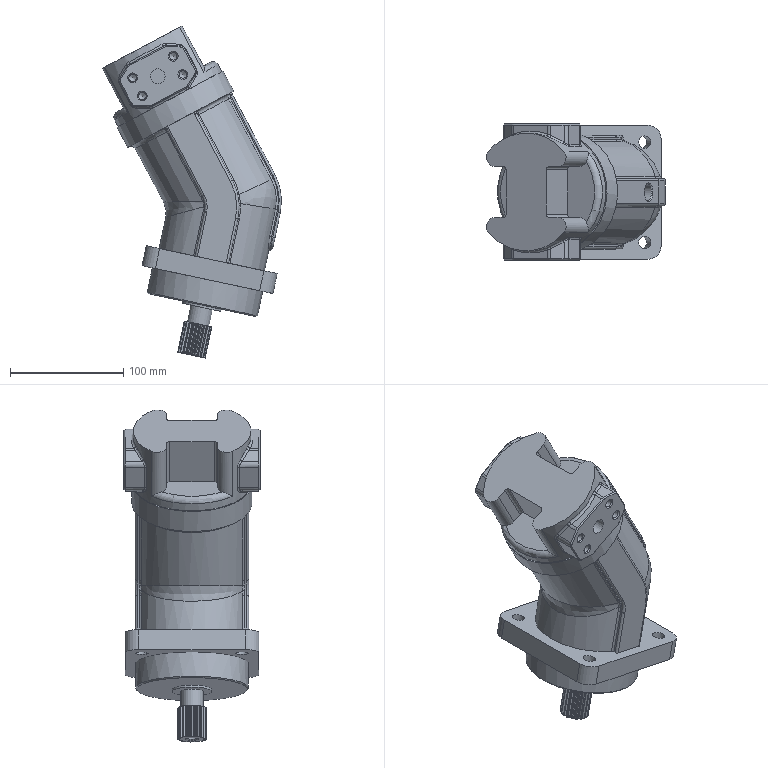Part | STEP file | HL4GZ-1.61.011 (hydraulic motor) | 1 solid | 385 faces | box 157.77 x 120 x 292.652 mm | volume 1969898 mm3 | cylinder 204 | plane 71 | spline 55 | cone 38 | torus 17 | commonest cylinder face diameters 0.5 x38 11.547 x38 4 x28 21.627 x19 25 x19 10 x17